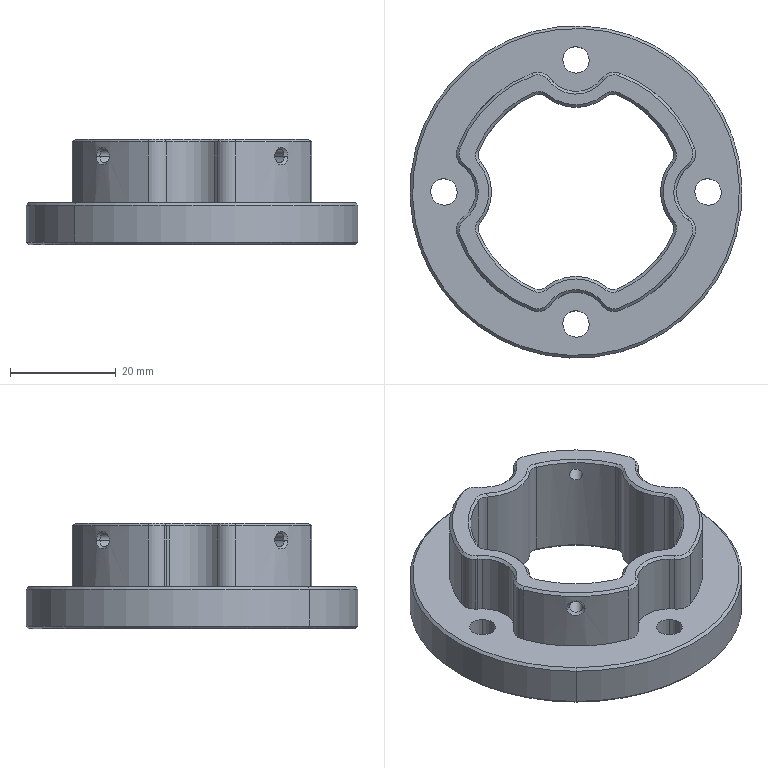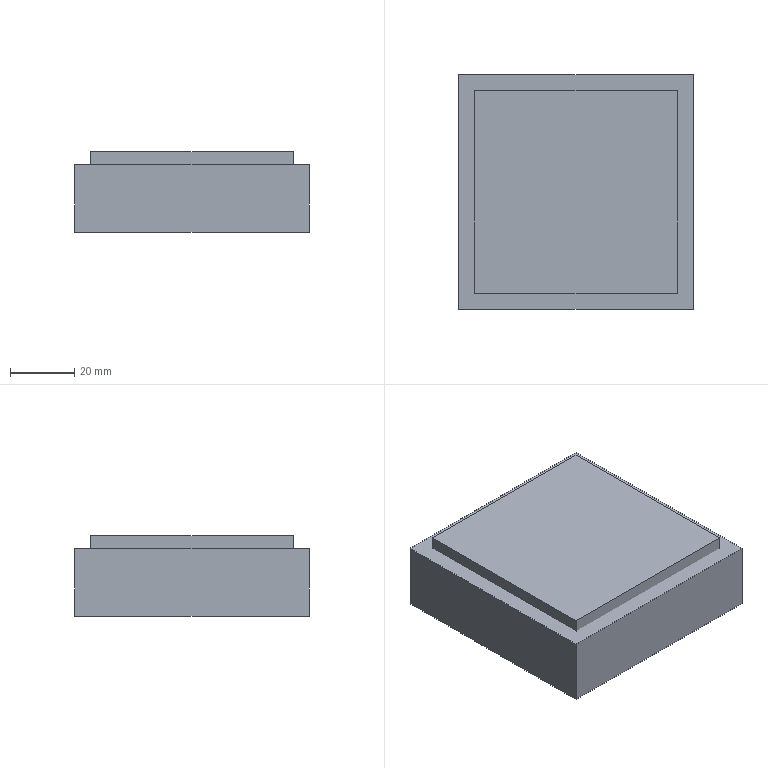CAM job | NX | 3-axis milling, drilling | part box 62.9 x 62.9 x 20 mm | stock box 72.9 x 72.9 x 25 mm
Tools:
number,name,description,diameter,corner_radius,flute_length,length,flutes
19,D80,Milling Tool-5 Parameters,80.0,0.0,50.0,75.0,2
15,D10,Milling Tool-5 Parameters,10.0,0.0,50.0,75.0,2
11,D4,Milling Tool-5 Parameters,4.0,0.0,50.0,75.0,2
1,D6A45,Milling Tool-5 Parameters,6.0,0.0,50.0,75.0,2
5,5.0ZT,Drilling Tool,5.0,0.0,35.0,50.0,2
Operations:
program,operation,operation_type,tool,method,geometry_group,spindle_rpm,surface_speed,feed_per_tooth,feed_cut,feed_plunge,cut_length_mm,path_length_mm,cut_time_min,machine_time_min
1,FLOOR_WALL,VolumeBased25DMillingOperation,D80,METHOD,A,6500.0,1633.0,0.1154,1500.0,100.0,164.9,218.9,0.1099,0.1153
1,ADAPTIVE_MILLING,CavityMilling,D10,METHOD,A,9500.0,298.0,0.1579,3000.0,1000.0,5430.268,5508.068,1.812,1.82
1,ADAPTIVE_MILLING_COPY,CavityMilling,D10,METHOD,A,9500.0,298.0,0.1579,3000.0,1000.0,7116.462,7323.489,3.253,3.273
1,CAVITY_MILL_COPY,CavityMilling,D4,METHOD,A,9500.0,179.0,0.1053,2000.0,1000.0,4876.787,9479.569,3.212,3.672
1,FLOOR_WALL_1,VolumeBased25DMillingOperation,D4,METHOD,A,9500.0,119.0,0.0658,1250.0,100.0,1090.233,1257.126,0.8722,0.8889
1,11,ZLevelMilling,D4,METHOD,A,9500.0,179.0,0.0632,1200.0,100.0,238.347,337.353,0.1986,0.2085
1,22,ZLevelMilling,D4,METHOD,A,9500.0,179.0,0.0632,1200.0,100.0,213.38,312.38,0.1778,0.1877
1,DRILLING,Operation,D6A45,METHOD,A,5000.0,94.0,0.035,350.0,0.0,22.4,244.247,0.064,0.0862
1,DRILLING_COPY_1_COPY,Operation,5.0ZT,METHOD,A,2000.0,20.0,0.05,200.0,0.0,56.009,311.464,0.28,0.3056
1,PLANAR_MILL_COPY_COPY_COPY_COPY_COPY_COPY_1,PlanarMilling,D6A45,METHOD,A,9500.0,179.0,0.0658,1250.0,100.0,297.392,425.491,0.2379,0.2507
1,PLANAR_MILL_COPY_COPY_COPY_COPY_COPY_COPY_1_COPY,PlanarMilling,D6A45,METHOD,A,9500.0,179.0,0.0658,1250.0,100.0,208.984,292.984,0.1672,0.1756
2,FLOOR_WALL_COPY,VolumeBased25DMillingOperation,D80,METHOD,B,6500.0,1633.0,0.1154,1500.0,100.0,804.5,1674.101,0.5363,0.6233
2,DRILLING_COPY,Operation,D6A45,METHOD,B,5000.0,94.0,0.035,350.0,0.0,22.4,220.247,0.064,0.0838
2,PLANAR_MILL_COPY_COPY_COPY_COPY_COPY_COPY_1_COPY_1,PlanarMilling,D6A45,METHOD,B,9500.0,179.0,0.0658,1250.0,100.0,336.337,474.787,0.2691,0.2829